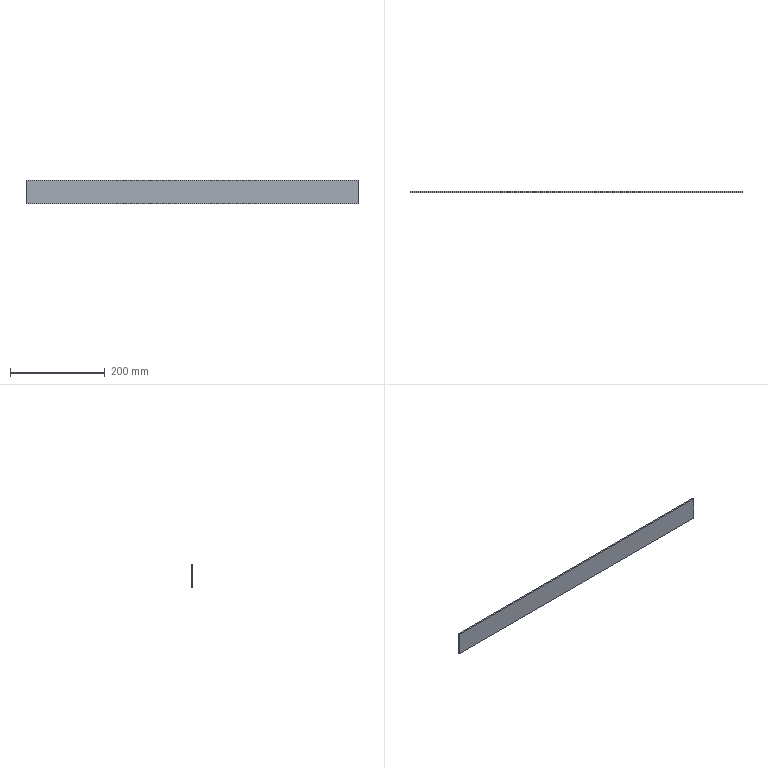Part | STEP file | Stair anti-slip strip_Default<As Machined> | 1 solid | 6 faces | box 700 x 3 x 50 mm | volume 105000 mm3 | plane 6
STEP:
#1=CARTESIAN_POINT('',(0.,0.,0.));
#2=DIRECTION('',(0.,0.,1.));
#3=DIRECTION('',(1.,0.,0.));
#4=AXIS2_PLACEMENT_3D('',#1,#2,#3);
#5=CARTESIAN_POINT('',(350.,0.,25.));
#6=VERTEX_POINT('',#5);
#7=CARTESIAN_POINT('',(350.,0.,-25.));
#8=VERTEX_POINT('',#7);
#9=CARTESIAN_POINT('',(350.,0.,25.));
#10=DIRECTION('',(0.,0.,-1.));
#11=VECTOR('',#10,1.);
#12=LINE('',#9,#11);
#13=CARTESIAN_POINT('',(350.,3.,25.));
#14=DIRECTION('',(-1.,0.,0.));
#15=DIRECTION('',(0.,0.,1.));
#16=AXIS2_PLACEMENT_3D('',#13,#14,#15);
#17=PLANE('',#16);
#18=CARTESIAN_POINT('',(0.,-3.));
#19=DIRECTION('',(-1.,0.));
#20=VECTOR('',#19,1.);
#21=LINE('',#18,#20);
#22=(GEOMETRIC_REPRESENTATION_CONTEXT(2)PARAMETRIC_REPRESENTATION_CONTEXT()REPRESENTATION_CONTEXT('',''));
#23=DEFINITIONAL_REPRESENTATION('',(#21),#22);
#24=PCURVE('',#17,#23);
#25=CARTESIAN_POINT('',(0.,0.,0.));
#26=DIRECTION('',(0.,-1.,0.));
#27=DIRECTION('',(0.,0.,-1.));
#28=AXIS2_PLACEMENT_3D('',#25,#26,#27);
#29=PLANE('',#28);
#30=CARTESIAN_POINT('',(-25.,350.));
#31=DIRECTION('',(1.,0.));
#32=VECTOR('',#31,1.);
#33=LINE('',#30,#32);
#34=(GEOMETRIC_REPRESENTATION_CONTEXT(2)PARAMETRIC_REPRESENTATION_CONTEXT()REPRESENTATION_CONTEXT('',''));
#35=DEFINITIONAL_REPRESENTATION('',(#33),#34);
#36=PCURVE('',#29,#35);
#37=SURFACE_CURVE('',#12,(#24,#36),.PCURVE_S1.);
#38=EDGE_CURVE('',#6,#8,#37,.T.);
#39=ORIENTED_EDGE('',*,*,#38,.T.);
#40=CARTESIAN_POINT('',(350.,3.,-25.));
#41=VERTEX_POINT('',#40);
#42=CARTESIAN_POINT('',(350.,3.,-25.));
#43=DIRECTION('',(0.,-1.,0.));
#44=VECTOR('',#43,1.);
#45=LINE('',#42,#44);
#46=CARTESIAN_POINT('',(-50.,0.));
#47=DIRECTION('',(0.,-1.));
#48=VECTOR('',#47,1.);
#49=LINE('',#46,#48);
#50=(GEOMETRIC_REPRESENTATION_CONTEXT(2)PARAMETRIC_REPRESENTATION_CONTEXT()REPRESENTATION_CONTEXT('',''));
#51=DEFINITIONAL_REPRESENTATION('',(#49),#50);
#52=PCURVE('',#17,#51);
#53=CARTESIAN_POINT('',(-350.,3.,-25.));
#54=DIRECTION('',(0.,0.,1.));
#55=DIRECTION('',(1.,0.,0.));
#56=AXIS2_PLACEMENT_3D('',#53,#54,#55);
#57=PLANE('',#56);
#58=CARTESIAN_POINT('',(700.,0.));
#59=DIRECTION('',(0.,-1.));
#60=VECTOR('',#59,1.);
#61=LINE('',#58,#60);
#62=(GEOMETRIC_REPRESENTATION_CONTEXT(2)PARAMETRIC_REPRESENTATION_CONTEXT()REPRESENTATION_CONTEXT('',''));
#63=DEFINITIONAL_REPRESENTATION('',(#61),#62);
#64=PCURVE('',#57,#63);
#65=SURFACE_CURVE('',#45,(#52,#64),.PCURVE_S1.);
#66=EDGE_CURVE('',#41,#8,#65,.T.);
#67=ORIENTED_EDGE('',*,*,#66,.F.);
#68=CARTESIAN_POINT('',(350.,3.,25.));
#69=VERTEX_POINT('',#68);
#70=CARTESIAN_POINT('',(350.,3.,25.));
#71=DIRECTION('',(0.,0.,-1.));
#72=VECTOR('',#71,1.);
#73=LINE('',#70,#72);
#74=CARTESIAN_POINT('',(0.,0.));
#75=DIRECTION('',(-1.,0.));
#76=VECTOR('',#75,1.);
#77=LINE('',#74,#76);
#78=(GEOMETRIC_REPRESENTATION_CONTEXT(2)PARAMETRIC_REPRESENTATION_CONTEXT()REPRESENTATION_CONTEXT('',''));
#79=DEFINITIONAL_REPRESENTATION('',(#77),#78);
#80=PCURVE('',#17,#79);
#81=CARTESIAN_POINT('',(0.,3.,0.));
#82=DIRECTION('',(0.,-1.,0.));
#83=DIRECTION('',(0.,0.,-1.));
#84=AXIS2_PLACEMENT_3D('',#81,#82,#83);
#85=PLANE('',#84);
#86=CARTESIAN_POINT('',(-25.,350.));
#87=DIRECTION('',(1.,0.));
#88=VECTOR('',#87,1.);
#89=LINE('',#86,#88);
#90=(GEOMETRIC_REPRESENTATION_CONTEXT(2)PARAMETRIC_REPRESENTATION_CONTEXT()REPRESENTATION_CONTEXT('',''));
#91=DEFINITIONAL_REPRESENTATION('',(#89),#90);
#92=PCURVE('',#85,#91);
#93=SURFACE_CURVE('',#73,(#80,#92),.PCURVE_S1.);
#94=EDGE_CURVE('',#69,#41,#93,.T.);
#95=ORIENTED_EDGE('',*,*,#94,.F.);
#96=CARTESIAN_POINT('',(350.,3.,25.));
#97=DIRECTION('',(0.,-1.,0.));
#98=VECTOR('',#97,1.);
#99=LINE('',#96,#98);
#100=CARTESIAN_POINT('',(0.,0.));
#101=DIRECTION('',(0.,-1.));
#102=VECTOR('',#101,1.);
#103=LINE('',#100,#102);
#104=(GEOMETRIC_REPRESENTATION_CONTEXT(2)PARAMETRIC_REPRESENTATION_CONTEXT()REPRESENTATION_CONTEXT('',''));
#105=DEFINITIONAL_REPRESENTATION('',(#103),#104);
#106=PCURVE('',#17,#105);
#107=CARTESIAN_POINT('',(-350.,3.,25.));
#108=DIRECTION('',(0.,0.,-1.));
#109=DIRECTION('',(-1.,0.,0.));
#110=AXIS2_PLACEMENT_3D('',#107,#108,#109);
#111=PLANE('',#110);
#112=CARTESIAN_POINT('',(-700.,0.));
#113=DIRECTION('',(0.,-1.));
#114=VECTOR('',#113,1.);
#115=LINE('',#112,#114);
#116=(GEOMETRIC_REPRESENTATION_CONTEXT(2)PARAMETRIC_REPRESENTATION_CONTEXT()REPRESENTATION_CONTEXT('',''));
#117=DEFINITIONAL_REPRESENTATION('',(#115),#116);
#118=PCURVE('',#111,#117);
#119=SURFACE_CURVE('',#99,(#106,#118),.PCURVE_S1.);
#120=EDGE_CURVE('',#69,#6,#119,.T.);
#121=ORIENTED_EDGE('',*,*,#120,.T.);
#122=EDGE_LOOP('',(#39,#67,#95,#121));
#123=FACE_BOUND('',#122,.T.);
#124=ADVANCED_FACE('',(#123),#17,.F.);
#125=CARTESIAN_POINT('',(-350.,0.,-25.));
#126=VERTEX_POINT('',#125);
#127=CARTESIAN_POINT('',(-350.,0.,-25.));
#128=DIRECTION('',(-1.,0.,0.));
#129=VECTOR('',#128,1.);
#130=LINE('',#127,#129);
#131=CARTESIAN_POINT('',(0.,-3.));
#132=DIRECTION('',(-1.,0.));
#133=VECTOR('',#132,1.);
#134=LINE('',#131,#133);
#135=(GEOMETRIC_REPRESENTATION_CONTEXT(2)PARAMETRIC_REPRESENTATION_CONTEXT()REPRESENTATION_CONTEXT('',''));
#136=DEFINITIONAL_REPRESENTATION('',(#134),#135);
#137=PCURVE('',#57,#136);
#138=CARTESIAN_POINT('',(25.,-350.));
#139=DIRECTION('',(0.,-1.));
#140=VECTOR('',#139,1.);
#141=LINE('',#138,#140);
#142=(GEOMETRIC_REPRESENTATION_CONTEXT(2)PARAMETRIC_REPRESENTATION_CONTEXT()REPRESENTATION_CONTEXT('',''));
#143=DEFINITIONAL_REPRESENTATION('',(#141),#142);
#144=PCURVE('',#29,#143);
#145=SURFACE_CURVE('',#130,(#137,#144),.PCURVE_S1.);
#146=EDGE_CURVE('',#8,#126,#145,.T.);
#147=ORIENTED_EDGE('',*,*,#146,.T.);
#148=CARTESIAN_POINT('',(-350.,3.,-25.));
#149=VERTEX_POINT('',#148);
#150=CARTESIAN_POINT('',(-350.,3.,-25.));
#151=DIRECTION('',(0.,-1.,0.));
#152=VECTOR('',#151,1.);
#153=LINE('',#150,#152);
#154=CARTESIAN_POINT('',(0.,0.));
#155=DIRECTION('',(0.,-1.));
#156=VECTOR('',#155,1.);
#157=LINE('',#154,#156);
#158=(GEOMETRIC_REPRESENTATION_CONTEXT(2)PARAMETRIC_REPRESENTATION_CONTEXT()REPRESENTATION_CONTEXT('',''));
#159=DEFINITIONAL_REPRESENTATION('',(#157),#158);
#160=PCURVE('',#57,#159);
#161=CARTESIAN_POINT('',(-350.,3.,25.));
#162=DIRECTION('',(1.,0.,0.));
#163=DIRECTION('',(0.,0.,-1.));
#164=AXIS2_PLACEMENT_3D('',#161,#162,#163);
#165=PLANE('',#164);
#166=CARTESIAN_POINT('',(50.,0.));
#167=DIRECTION('',(0.,-1.));
#168=VECTOR('',#167,1.);
#169=LINE('',#166,#168);
#170=(GEOMETRIC_REPRESENTATION_CONTEXT(2)PARAMETRIC_REPRESENTATION_CONTEXT()REPRESENTATION_CONTEXT('',''));
#171=DEFINITIONAL_REPRESENTATION('',(#169),#170);
#172=PCURVE('',#165,#171);
#173=SURFACE_CURVE('',#153,(#160,#172),.PCURVE_S1.);
#174=EDGE_CURVE('',#149,#126,#173,.T.);
#175=ORIENTED_EDGE('',*,*,#174,.F.);
#176=CARTESIAN_POINT('',(-350.,3.,-25.));
#177=DIRECTION('',(-1.,0.,0.));
#178=VECTOR('',#177,1.);
#179=LINE('',#176,#178);
#180=CARTESIAN_POINT('',(0.,0.));
#181=DIRECTION('',(-1.,0.));
#182=VECTOR('',#181,1.);
#183=LINE('',#180,#182);
#184=(GEOMETRIC_REPRESENTATION_CONTEXT(2)PARAMETRIC_REPRESENTATION_CONTEXT()REPRESENTATION_CONTEXT('',''));
#185=DEFINITIONAL_REPRESENTATION('',(#183),#184);
#186=PCURVE('',#57,#185);
#187=CARTESIAN_POINT('',(25.,-350.));
#188=DIRECTION('',(0.,-1.));
#189=VECTOR('',#188,1.);
#190=LINE('',#187,#189);
#191=(GEOMETRIC_REPRESENTATION_CONTEXT(2)PARAMETRIC_REPRESENTATION_CONTEXT()REPRESENTATION_CONTEXT('',''));
#192=DEFINITIONAL_REPRESENTATION('',(#190),#191);
#193=PCURVE('',#85,#192);
#194=SURFACE_CURVE('',#179,(#186,#193),.PCURVE_S1.);
#195=EDGE_CURVE('',#41,#149,#194,.T.);
#196=ORIENTED_EDGE('',*,*,#195,.F.);
#197=ORIENTED_EDGE('',*,*,#66,.T.);
#198=EDGE_LOOP('',(#147,#175,#196,#197));
#199=FACE_BOUND('',#198,.T.);
#200=ADVANCED_FACE('',(#199),#57,.F.);
#201=CARTESIAN_POINT('',(-350.,0.,25.));
#202=VERTEX_POINT('',#201);
#203=CARTESIAN_POINT('',(-350.,0.,25.));
#204=DIRECTION('',(0.,0.,1.));
#205=VECTOR('',#204,1.);
#206=LINE('',#203,#205);
#207=CARTESIAN_POINT('',(0.,-3.));
#208=DIRECTION('',(-1.,0.));
#209=VECTOR('',#208,1.);
#210=LINE('',#207,#209);
#211=(GEOMETRIC_REPRESENTATION_CONTEXT(2)PARAMETRIC_REPRESENTATION_CONTEXT()REPRESENTATION_CONTEXT('',''));
#212=DEFINITIONAL_REPRESENTATION('',(#210),#211);
#213=PCURVE('',#165,#212);
#214=CARTESIAN_POINT('',(-25.,-350.));
#215=DIRECTION('',(-1.,0.));
#216=VECTOR('',#215,1.);
#217=LINE('',#214,#216);
#218=(GEOMETRIC_REPRESENTATION_CONTEXT(2)PARAMETRIC_REPRESENTATION_CONTEXT()REPRESENTATION_CONTEXT('',''));
#219=DEFINITIONAL_REPRESENTATION('',(#217),#218);
#220=PCURVE('',#29,#219);
#221=SURFACE_CURVE('',#206,(#213,#220),.PCURVE_S1.);
#222=EDGE_CURVE('',#126,#202,#221,.T.);
#223=ORIENTED_EDGE('',*,*,#222,.T.);
#224=CARTESIAN_POINT('',(-350.,3.,25.));
#225=VERTEX_POINT('',#224);
#226=CARTESIAN_POINT('',(-350.,3.,25.));
#227=DIRECTION('',(0.,-1.,0.));
#228=VECTOR('',#227,1.);
#229=LINE('',#226,#228);
#230=CARTESIAN_POINT('',(0.,0.));
#231=DIRECTION('',(0.,-1.));
#232=VECTOR('',#231,1.);
#233=LINE('',#230,#232);
#234=(GEOMETRIC_REPRESENTATION_CONTEXT(2)PARAMETRIC_REPRESENTATION_CONTEXT()REPRESENTATION_CONTEXT('',''));
#235=DEFINITIONAL_REPRESENTATION('',(#233),#234);
#236=PCURVE('',#165,#235);
#237=CARTESIAN_POINT('',(0.,0.));
#238=DIRECTION('',(0.,-1.));
#239=VECTOR('',#238,1.);
#240=LINE('',#237,#239);
#241=(GEOMETRIC_REPRESENTATION_CONTEXT(2)PARAMETRIC_REPRESENTATION_CONTEXT()REPRESENTATION_CONTEXT('',''));
#242=DEFINITIONAL_REPRESENTATION('',(#240),#241);
#243=PCURVE('',#111,#242);
#244=SURFACE_CURVE('',#229,(#236,#243),.PCURVE_S1.);
#245=EDGE_CURVE('',#225,#202,#244,.T.);
#246=ORIENTED_EDGE('',*,*,#245,.F.);
#247=CARTESIAN_POINT('',(-350.,3.,25.));
#248=DIRECTION('',(0.,0.,1.));
#249=VECTOR('',#248,1.);
#250=LINE('',#247,#249);
#251=CARTESIAN_POINT('',(0.,0.));
#252=DIRECTION('',(-1.,0.));
#253=VECTOR('',#252,1.);
#254=LINE('',#251,#253);
#255=(GEOMETRIC_REPRESENTATION_CONTEXT(2)PARAMETRIC_REPRESENTATION_CONTEXT()REPRESENTATION_CONTEXT('',''));
#256=DEFINITIONAL_REPRESENTATION('',(#254),#255);
#257=PCURVE('',#165,#256);
#258=CARTESIAN_POINT('',(-25.,-350.));
#259=DIRECTION('',(-1.,0.));
#260=VECTOR('',#259,1.);
#261=LINE('',#258,#260);
#262=(GEOMETRIC_REPRESENTATION_CONTEXT(2)PARAMETRIC_REPRESENTATION_CONTEXT()REPRESENTATION_CONTEXT('',''));
#263=DEFINITIONAL_REPRESENTATION('',(#261),#262);
#264=PCURVE('',#85,#263);
#265=SURFACE_CURVE('',#250,(#257,#264),.PCURVE_S1.);
#266=EDGE_CURVE('',#149,#225,#265,.T.);
#267=ORIENTED_EDGE('',*,*,#266,.F.);
#268=ORIENTED_EDGE('',*,*,#174,.T.);
#269=EDGE_LOOP('',(#223,#246,#267,#268));
#270=FACE_BOUND('',#269,.T.);
#271=ADVANCED_FACE('',(#270),#165,.F.);
#272=CARTESIAN_POINT('',(-350.,0.,25.));
#273=DIRECTION('',(1.,0.,0.));
#274=VECTOR('',#273,1.);
#275=LINE('',#272,#274);
#276=CARTESIAN_POINT('',(0.,-3.));
#277=DIRECTION('',(-1.,0.));
#278=VECTOR('',#277,1.);
#279=LINE('',#276,#278);
#280=(GEOMETRIC_REPRESENTATION_CONTEXT(2)PARAMETRIC_REPRESENTATION_CONTEXT()REPRESENTATION_CONTEXT('',''));
#281=DEFINITIONAL_REPRESENTATION('',(#279),#280);
#282=PCURVE('',#111,#281);
#283=CARTESIAN_POINT('',(-25.,-350.));
#284=DIRECTION('',(0.,1.));
#285=VECTOR('',#284,1.);
#286=LINE('',#283,#285);
#287=(GEOMETRIC_REPRESENTATION_CONTEXT(2)PARAMETRIC_REPRESENTATION_CONTEXT()REPRESENTATION_CONTEXT('',''));
#288=DEFINITIONAL_REPRESENTATION('',(#286),#287);
#289=PCURVE('',#29,#288);
#290=SURFACE_CURVE('',#275,(#282,#289),.PCURVE_S1.);
#291=EDGE_CURVE('',#202,#6,#290,.T.);
#292=ORIENTED_EDGE('',*,*,#291,.T.);
#293=ORIENTED_EDGE('',*,*,#120,.F.);
#294=CARTESIAN_POINT('',(-350.,3.,25.));
#295=DIRECTION('',(1.,0.,0.));
#296=VECTOR('',#295,1.);
#297=LINE('',#294,#296);
#298=CARTESIAN_POINT('',(0.,0.));
#299=DIRECTION('',(-1.,0.));
#300=VECTOR('',#299,1.);
#301=LINE('',#298,#300);
#302=(GEOMETRIC_REPRESENTATION_CONTEXT(2)PARAMETRIC_REPRESENTATION_CONTEXT()REPRESENTATION_CONTEXT('',''));
#303=DEFINITIONAL_REPRESENTATION('',(#301),#302);
#304=PCURVE('',#111,#303);
#305=CARTESIAN_POINT('',(-25.,-350.));
#306=DIRECTION('',(0.,1.));
#307=VECTOR('',#306,1.);
#308=LINE('',#305,#307);
#309=(GEOMETRIC_REPRESENTATION_CONTEXT(2)PARAMETRIC_REPRESENTATION_CONTEXT()REPRESENTATION_CONTEXT('',''));
#310=DEFINITIONAL_REPRESENTATION('',(#308),#309);
#311=PCURVE('',#85,#310);
#312=SURFACE_CURVE('',#297,(#304,#311),.PCURVE_S1.);
#313=EDGE_CURVE('',#225,#69,#312,.T.);
#314=ORIENTED_EDGE('',*,*,#313,.F.);
#315=ORIENTED_EDGE('',*,*,#245,.T.);
#316=EDGE_LOOP('',(#292,#293,#314,#315));
#317=FACE_BOUND('',#316,.T.);
#318=ADVANCED_FACE('',(#317),#111,.F.);
#319=ORIENTED_EDGE('',*,*,#94,.T.);
#320=ORIENTED_EDGE('',*,*,#195,.T.);
#321=ORIENTED_EDGE('',*,*,#266,.T.);
#322=ORIENTED_EDGE('',*,*,#313,.T.);
#323=EDGE_LOOP('',(#319,#320,#321,#322));
#324=FACE_BOUND('',#323,.T.);
#325=ADVANCED_FACE('',(#324),#85,.F.);
#326=ORIENTED_EDGE('',*,*,#38,.F.);
#327=ORIENTED_EDGE('',*,*,#291,.F.);
#328=ORIENTED_EDGE('',*,*,#222,.F.);
#329=ORIENTED_EDGE('',*,*,#146,.F.);
#330=EDGE_LOOP('',(#326,#327,#328,#329));
#331=FACE_BOUND('',#330,.T.);
#332=ADVANCED_FACE('',(#331),#29,.T.);
#333=CLOSED_SHELL('',(#124,#200,#271,#318,#325,#332));
#334=MANIFOLD_SOLID_BREP('',#333);
#335=(LENGTH_UNIT()NAMED_UNIT(*)SI_UNIT(.MILLI.,.METRE.));
#336=UNCERTAINTY_MEASURE_WITH_UNIT(LENGTH_MEASURE(0.0000001),#335,'','');
#337=(NAMED_UNIT(*)PLANE_ANGLE_UNIT()SI_UNIT($,.RADIAN.));
#338=(NAMED_UNIT(*)SI_UNIT($,.STERADIAN.)SOLID_ANGLE_UNIT());
#339=(GEOMETRIC_REPRESENTATION_CONTEXT(3)GLOBAL_UNCERTAINTY_ASSIGNED_CONTEXT((#336))GLOBAL_UNIT_ASSIGNED_CONTEXT((#335,#337,#338))REPRESENTATION_CONTEXT('',''));
#340=ADVANCED_BREP_SHAPE_REPRESENTATION('',(#4,#334),#339);